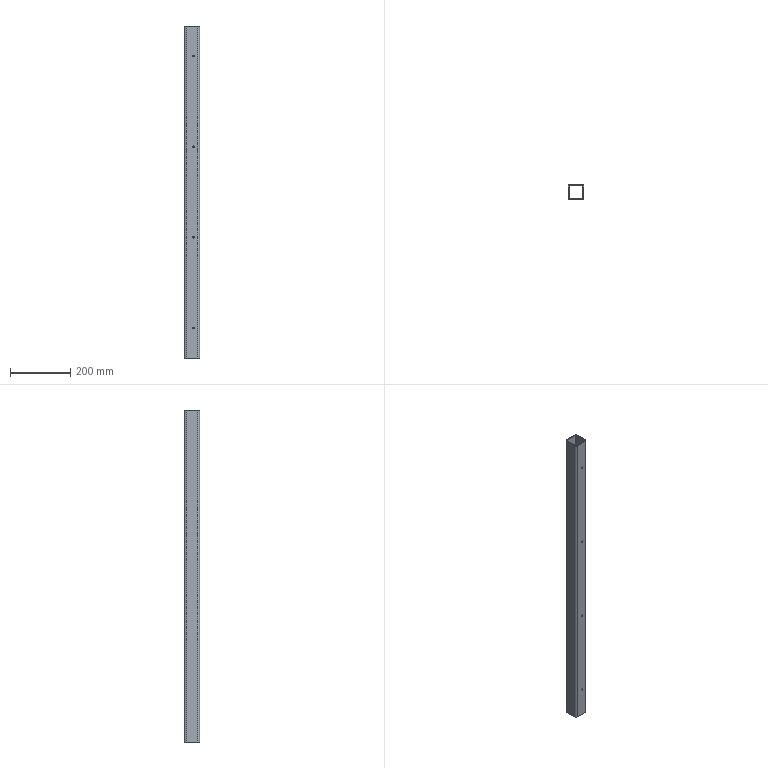Part | SolidWorks | features HoleWzd 1, WeldMemberFeat 1, WeldmentFeature 1 | 1 solid | 26 faces | box 50 x 50 x 1100 mm | volume 594670 mm3 | cylinder 16 | plane 10 | commonest cylinder face diameters 5 x8 6 x4 12 x4
STEP:
#1=CARTESIAN_POINT('',(5.,-22.,-102.5));
#2=VERTEX_POINT('',#1);
#3=CARTESIAN_POINT('',(5.,-22.,-97.5));
#4=VERTEX_POINT('',#3);
#5=CARTESIAN_POINT('',(5.,-22.,-100.));
#6=DIRECTION('',(0.,1.,0.));
#7=DIRECTION('',(0.,0.,1.));
#8=AXIS2_PLACEMENT_3D('',#5,#6,#7);
#9=CIRCLE('',#8,2.5);
#10=EDGE_CURVE('',#2,#4,#9,.T.);
#11=ORIENTED_EDGE('',*,*,#10,.T.);
#12=CARTESIAN_POINT('',(5.,-25.,-97.5));
#13=VERTEX_POINT('',#12);
#14=CARTESIAN_POINT('',(5.,-25.,-97.5));
#15=DIRECTION('',(0.,-1.,0.));
#16=VECTOR('',#15,1000.);
#17=LINE('',#14,#16);
#18=EDGE_CURVE('',#4,#13,#17,.T.);
#19=ORIENTED_EDGE('',*,*,#18,.T.);
#20=CARTESIAN_POINT('',(5.,-25.,-102.5));
#21=VERTEX_POINT('',#20);
#22=CARTESIAN_POINT('',(5.,-25.,-100.));
#23=DIRECTION('',(0.,-1.,0.));
#24=DIRECTION('',(0.,0.,-1.));
#25=AXIS2_PLACEMENT_3D('',#22,#23,#24);
#26=CIRCLE('',#25,2.5);
#27=EDGE_CURVE('',#13,#21,#26,.T.);
#28=ORIENTED_EDGE('',*,*,#27,.T.);
#29=CARTESIAN_POINT('',(5.,-25.,-102.5));
#30=DIRECTION('',(0.,-1.,0.));
#31=VECTOR('',#30,1000.);
#32=LINE('',#29,#31);
#33=EDGE_CURVE('',#2,#21,#32,.T.);
#34=ORIENTED_EDGE('',*,*,#33,.F.);
#35=EDGE_LOOP('',(#11,#19,#28,#34));
#36=FACE_OUTER_BOUND('',#35,.T.);
#37=CARTESIAN_POINT('',(5.,-25.,-100.));
#38=DIRECTION('',(0.,-1.,0.));
#39=DIRECTION('',(0.,0.,-1.));
#40=AXIS2_PLACEMENT_3D('',#37,#38,#39);
#41=CYLINDRICAL_SURFACE('',#40,2.5);
#42=ADVANCED_FACE('',(#36),#41,.F.);
#43=CARTESIAN_POINT('',(5.,-22.,-402.5));
#44=VERTEX_POINT('',#43);
#45=CARTESIAN_POINT('',(5.,-22.,-397.5));
#46=VERTEX_POINT('',#45);
#47=CARTESIAN_POINT('',(5.,-22.,-400.));
#48=DIRECTION('',(0.,1.,0.));
#49=DIRECTION('',(0.,0.,1.));
#50=AXIS2_PLACEMENT_3D('',#47,#48,#49);
#51=CIRCLE('',#50,2.5);
#52=EDGE_CURVE('',#44,#46,#51,.T.);
#53=ORIENTED_EDGE('',*,*,#52,.T.);
#54=CARTESIAN_POINT('',(5.,-25.,-397.5));
#55=VERTEX_POINT('',#54);
#56=CARTESIAN_POINT('',(5.,-25.,-397.5));
#57=DIRECTION('',(0.,-1.,0.));
#58=VECTOR('',#57,1000.);
#59=LINE('',#56,#58);
#60=EDGE_CURVE('',#46,#55,#59,.T.);
#61=ORIENTED_EDGE('',*,*,#60,.T.);
#62=CARTESIAN_POINT('',(5.,-25.,-402.5));
#63=VERTEX_POINT('',#62);
#64=CARTESIAN_POINT('',(5.,-25.,-400.));
#65=DIRECTION('',(0.,-1.,0.));
#66=DIRECTION('',(0.,0.,-1.));
#67=AXIS2_PLACEMENT_3D('',#64,#65,#66);
#68=CIRCLE('',#67,2.5);
#69=EDGE_CURVE('',#55,#63,#68,.T.);
#70=ORIENTED_EDGE('',*,*,#69,.T.);
#71=CARTESIAN_POINT('',(5.,-25.,-402.5));
#72=DIRECTION('',(0.,-1.,0.));
#73=VECTOR('',#72,1000.);
#74=LINE('',#71,#73);
#75=EDGE_CURVE('',#44,#63,#74,.T.);
#76=ORIENTED_EDGE('',*,*,#75,.F.);
#77=EDGE_LOOP('',(#53,#61,#70,#76));
#78=FACE_OUTER_BOUND('',#77,.T.);
#79=CARTESIAN_POINT('',(5.,-25.,-400.));
#80=DIRECTION('',(0.,-1.,0.));
#81=DIRECTION('',(0.,0.,-1.));
#82=AXIS2_PLACEMENT_3D('',#79,#80,#81);
#83=CYLINDRICAL_SURFACE('',#82,2.5);
#84=ADVANCED_FACE('',(#78),#83,.F.);
#85=CARTESIAN_POINT('',(5.,-22.,-702.5));
#86=VERTEX_POINT('',#85);
#87=CARTESIAN_POINT('',(5.,-22.,-697.5));
#88=VERTEX_POINT('',#87);
#89=CARTESIAN_POINT('',(5.,-22.,-700.));
#90=DIRECTION('',(0.,1.,0.));
#91=DIRECTION('',(0.,0.,1.));
#92=AXIS2_PLACEMENT_3D('',#89,#90,#91);
#93=CIRCLE('',#92,2.5);
#94=EDGE_CURVE('',#86,#88,#93,.T.);
#95=ORIENTED_EDGE('',*,*,#94,.T.);
#96=CARTESIAN_POINT('',(5.,-25.,-697.5));
#97=VERTEX_POINT('',#96);
#98=CARTESIAN_POINT('',(5.,-25.,-697.5));
#99=DIRECTION('',(0.,-1.,0.));
#100=VECTOR('',#99,1000.);
#101=LINE('',#98,#100);
#102=EDGE_CURVE('',#88,#97,#101,.T.);
#103=ORIENTED_EDGE('',*,*,#102,.T.);
#104=CARTESIAN_POINT('',(5.,-25.,-702.5));
#105=VERTEX_POINT('',#104);
#106=CARTESIAN_POINT('',(5.,-25.,-700.));
#107=DIRECTION('',(0.,-1.,0.));
#108=DIRECTION('',(0.,0.,-1.));
#109=AXIS2_PLACEMENT_3D('',#106,#107,#108);
#110=CIRCLE('',#109,2.5);
#111=EDGE_CURVE('',#97,#105,#110,.T.);
#112=ORIENTED_EDGE('',*,*,#111,.T.);
#113=CARTESIAN_POINT('',(5.,-25.,-702.5));
#114=DIRECTION('',(0.,-1.,0.));
#115=VECTOR('',#114,1000.);
#116=LINE('',#113,#115);
#117=EDGE_CURVE('',#86,#105,#116,.T.);
#118=ORIENTED_EDGE('',*,*,#117,.F.);
#119=EDGE_LOOP('',(#95,#103,#112,#118));
#120=FACE_OUTER_BOUND('',#119,.T.);
#121=CARTESIAN_POINT('',(5.,-25.,-700.));
#122=DIRECTION('',(0.,-1.,0.));
#123=DIRECTION('',(0.,0.,-1.));
#124=AXIS2_PLACEMENT_3D('',#121,#122,#123);
#125=CYLINDRICAL_SURFACE('',#124,2.5);
#126=ADVANCED_FACE('',(#120),#125,.F.);
#127=CARTESIAN_POINT('',(5.,-22.,-1002.5));
#128=VERTEX_POINT('',#127);
#129=CARTESIAN_POINT('',(5.,-22.,-997.5));
#130=VERTEX_POINT('',#129);
#131=CARTESIAN_POINT('',(5.,-22.,-1000.));
#132=DIRECTION('',(0.,1.,0.));
#133=DIRECTION('',(0.,0.,1.));
#134=AXIS2_PLACEMENT_3D('',#131,#132,#133);
#135=CIRCLE('',#134,2.5);
#136=EDGE_CURVE('',#128,#130,#135,.T.);
#137=ORIENTED_EDGE('',*,*,#136,.T.);
#138=CARTESIAN_POINT('',(5.,-25.,-997.5));
#139=VERTEX_POINT('',#138);
#140=CARTESIAN_POINT('',(5.,-25.,-997.5));
#141=DIRECTION('',(0.,-1.,0.));
#142=VECTOR('',#141,1000.);
#143=LINE('',#140,#142);
#144=EDGE_CURVE('',#130,#139,#143,.T.);
#145=ORIENTED_EDGE('',*,*,#144,.T.);
#146=CARTESIAN_POINT('',(5.,-25.,-1002.5));
#147=VERTEX_POINT('',#146);
#148=CARTESIAN_POINT('',(5.,-25.,-1000.));
#149=DIRECTION('',(0.,-1.,0.));
#150=DIRECTION('',(0.,0.,-1.));
#151=AXIS2_PLACEMENT_3D('',#148,#149,#150);
#152=CIRCLE('',#151,2.5);
#153=EDGE_CURVE('',#139,#147,#152,.T.);
#154=ORIENTED_EDGE('',*,*,#153,.T.);
#155=CARTESIAN_POINT('',(5.,-25.,-1002.5));
#156=DIRECTION('',(0.,-1.,0.));
#157=VECTOR('',#156,1000.);
#158=LINE('',#155,#157);
#159=EDGE_CURVE('',#128,#147,#158,.T.);
#160=ORIENTED_EDGE('',*,*,#159,.F.);
#161=EDGE_LOOP('',(#137,#145,#154,#160));
#162=FACE_OUTER_BOUND('',#161,.T.);
#163=CARTESIAN_POINT('',(5.,-25.,-1000.));
#164=DIRECTION('',(0.,-1.,0.));
#165=DIRECTION('',(0.,0.,-1.));
#166=AXIS2_PLACEMENT_3D('',#163,#164,#165);
#167=CYLINDRICAL_SURFACE('',#166,2.5);
#168=ADVANCED_FACE('',(#162),#167,.F.);
#169=CARTESIAN_POINT('',(-25.,19.,0.));
#170=VERTEX_POINT('',#169);
#171=CARTESIAN_POINT('',(-19.,25.,0.));
#172=VERTEX_POINT('',#171);
#173=CARTESIAN_POINT('',(-19.,19.,0.));
#174=DIRECTION('',(0.,0.,-1.));
#175=DIRECTION('',(-1.,0.,0.));
#176=AXIS2_PLACEMENT_3D('',#173,#174,#175);
#177=CIRCLE('',#176,6.);
#178=EDGE_CURVE('',#170,#172,#177,.T.);
#179=ORIENTED_EDGE('',*,*,#178,.T.);
#180=CARTESIAN_POINT('',(-19.,25.,-1100.));
#181=VERTEX_POINT('',#180);
#182=CARTESIAN_POINT('',(-19.,25.,-1100.));
#183=DIRECTION('',(0.,0.,1.));
#184=VECTOR('',#183,1000.);
#185=LINE('',#182,#184);
#186=EDGE_CURVE('',#181,#172,#185,.T.);
#187=ORIENTED_EDGE('',*,*,#186,.F.);
#188=CARTESIAN_POINT('',(-25.,19.,-1100.));
#189=VERTEX_POINT('',#188);
#190=CARTESIAN_POINT('',(-19.,19.,-1100.));
#191=DIRECTION('',(0.,0.,-1.));
#192=DIRECTION('',(-1.,0.,0.));
#193=AXIS2_PLACEMENT_3D('',#190,#191,#192);
#194=CIRCLE('',#193,6.);
#195=EDGE_CURVE('',#189,#181,#194,.T.);
#196=ORIENTED_EDGE('',*,*,#195,.F.);
#197=CARTESIAN_POINT('',(-25.,19.,-1100.));
#198=DIRECTION('',(0.,0.,1.));
#199=VECTOR('',#198,1000.);
#200=LINE('',#197,#199);
#201=EDGE_CURVE('',#189,#170,#200,.T.);
#202=ORIENTED_EDGE('',*,*,#201,.T.);
#203=EDGE_LOOP('',(#179,#187,#196,#202));
#204=FACE_OUTER_BOUND('',#203,.T.);
#205=CARTESIAN_POINT('',(-19.,19.,-1100.));
#206=DIRECTION('',(0.,0.,1.));
#207=DIRECTION('',(1.,0.,0.));
#208=AXIS2_PLACEMENT_3D('',#205,#206,#207);
#209=CYLINDRICAL_SURFACE('',#208,6.);
#210=ADVANCED_FACE('',(#204),#209,.T.);
#211=CARTESIAN_POINT('',(19.,25.,0.));
#212=VERTEX_POINT('',#211);
#213=CARTESIAN_POINT('',(-19.,25.,0.));
#214=DIRECTION('',(1.,0.,0.));
#215=VECTOR('',#214,1000.);
#216=LINE('',#213,#215);
#217=EDGE_CURVE('',#172,#212,#216,.T.);
#218=ORIENTED_EDGE('',*,*,#217,.T.);
#219=CARTESIAN_POINT('',(19.,25.,-1100.));
#220=VERTEX_POINT('',#219);
#221=CARTESIAN_POINT('',(19.,25.,-1100.));
#222=DIRECTION('',(0.,0.,1.));
#223=VECTOR('',#222,1000.);
#224=LINE('',#221,#223);
#225=EDGE_CURVE('',#220,#212,#224,.T.);
#226=ORIENTED_EDGE('',*,*,#225,.F.);
#227=CARTESIAN_POINT('',(-19.,25.,-1100.));
#228=DIRECTION('',(1.,0.,0.));
#229=VECTOR('',#228,1000.);
#230=LINE('',#227,#229);
#231=EDGE_CURVE('',#181,#220,#230,.T.);
#232=ORIENTED_EDGE('',*,*,#231,.F.);
#233=ORIENTED_EDGE('',*,*,#186,.T.);
#234=EDGE_LOOP('',(#218,#226,#232,#233));
#235=FACE_OUTER_BOUND('',#234,.T.);
#236=CARTESIAN_POINT('',(-19.,25.,-1100.));
#237=DIRECTION('',(0.,-1.,0.));
#238=DIRECTION('',(0.,0.,-1.));
#239=AXIS2_PLACEMENT_3D('',#236,#237,#238);
#240=PLANE('',#239);
#241=ADVANCED_FACE('',(#235),#240,.F.);
#242=CARTESIAN_POINT('',(25.,19.,0.));
#243=VERTEX_POINT('',#242);
#244=CARTESIAN_POINT('',(19.,19.,0.));
#245=DIRECTION('',(0.,0.,-1.));
#246=DIRECTION('',(-1.,0.,0.));
#247=AXIS2_PLACEMENT_3D('',#244,#245,#246);
#248=CIRCLE('',#247,6.);
#249=EDGE_CURVE('',#212,#243,#248,.T.);
#250=ORIENTED_EDGE('',*,*,#249,.T.);
#251=CARTESIAN_POINT('',(25.,19.,-1100.));
#252=VERTEX_POINT('',#251);
#253=CARTESIAN_POINT('',(25.,19.,-1100.));
#254=DIRECTION('',(0.,0.,1.));
#255=VECTOR('',#254,1000.);
#256=LINE('',#253,#255);
#257=EDGE_CURVE('',#252,#243,#256,.T.);
#258=ORIENTED_EDGE('',*,*,#257,.F.);
#259=CARTESIAN_POINT('',(19.,19.,-1100.));
#260=DIRECTION('',(0.,0.,-1.));
#261=DIRECTION('',(-1.,0.,0.));
#262=AXIS2_PLACEMENT_3D('',#259,#260,#261);
#263=CIRCLE('',#262,6.);
#264=EDGE_CURVE('',#220,#252,#263,.T.);
#265=ORIENTED_EDGE('',*,*,#264,.F.);
#266=ORIENTED_EDGE('',*,*,#225,.T.);
#267=EDGE_LOOP('',(#250,#258,#265,#266));
#268=FACE_OUTER_BOUND('',#267,.T.);
#269=CARTESIAN_POINT('',(19.,19.,-1100.));
#270=DIRECTION('',(0.,0.,1.));
#271=DIRECTION('',(1.,0.,0.));
#272=AXIS2_PLACEMENT_3D('',#269,#270,#271);
#273=CYLINDRICAL_SURFACE('',#272,6.);
#274=ADVANCED_FACE('',(#268),#273,.T.);
#275=CARTESIAN_POINT('',(25.,-19.,0.));
#276=VERTEX_POINT('',#275);
#277=CARTESIAN_POINT('',(25.,-19.,0.));
#278=DIRECTION('',(0.,-1.,0.));
#279=VECTOR('',#278,1000.);
#280=LINE('',#277,#279);
#281=EDGE_CURVE('',#243,#276,#280,.T.);
#282=ORIENTED_EDGE('',*,*,#281,.T.);
#283=CARTESIAN_POINT('',(25.,-19.,-1100.));
#284=VERTEX_POINT('',#283);
#285=CARTESIAN_POINT('',(25.,-19.,-1100.));
#286=DIRECTION('',(0.,0.,1.));
#287=VECTOR('',#286,1000.);
#288=LINE('',#285,#287);
#289=EDGE_CURVE('',#284,#276,#288,.T.);
#290=ORIENTED_EDGE('',*,*,#289,.F.);
#291=CARTESIAN_POINT('',(25.,-19.,-1100.));
#292=DIRECTION('',(0.,-1.,0.));
#293=VECTOR('',#292,1000.);
#294=LINE('',#291,#293);
#295=EDGE_CURVE('',#252,#284,#294,.T.);
#296=ORIENTED_EDGE('',*,*,#295,.F.);
#297=ORIENTED_EDGE('',*,*,#257,.T.);
#298=EDGE_LOOP('',(#282,#290,#296,#297));
#299=FACE_OUTER_BOUND('',#298,.T.);
#300=CARTESIAN_POINT('',(25.,-19.,-1100.));
#301=DIRECTION('',(-1.,0.,0.));
#302=DIRECTION('',(0.,0.,1.));
#303=AXIS2_PLACEMENT_3D('',#300,#301,#302);
#304=PLANE('',#303);
#305=ADVANCED_FACE('',(#299),#304,.F.);
#306=CARTESIAN_POINT('',(19.,-25.,0.));
#307=VERTEX_POINT('',#306);
#308=CARTESIAN_POINT('',(19.,-19.,0.));
#309=DIRECTION('',(0.,0.,-1.));
#310=DIRECTION('',(-1.,0.,0.));
#311=AXIS2_PLACEMENT_3D('',#308,#309,#310);
#312=CIRCLE('',#311,6.);
#313=EDGE_CURVE('',#276,#307,#312,.T.);
#314=ORIENTED_EDGE('',*,*,#313,.T.);
#315=CARTESIAN_POINT('',(19.,-25.,-1100.));
#316=VERTEX_POINT('',#315);
#317=CARTESIAN_POINT('',(19.,-25.,-1100.));
#318=DIRECTION('',(0.,0.,1.));
#319=VECTOR('',#318,1000.);
#320=LINE('',#317,#319);
#321=EDGE_CURVE('',#316,#307,#320,.T.);
#322=ORIENTED_EDGE('',*,*,#321,.F.);
#323=CARTESIAN_POINT('',(19.,-19.,-1100.));
#324=DIRECTION('',(0.,0.,-1.));
#325=DIRECTION('',(-1.,0.,0.));
#326=AXIS2_PLACEMENT_3D('',#323,#324,#325);
#327=CIRCLE('',#326,6.);
#328=EDGE_CURVE('',#284,#316,#327,.T.);
#329=ORIENTED_EDGE('',*,*,#328,.F.);
#330=ORIENTED_EDGE('',*,*,#289,.T.);
#331=EDGE_LOOP('',(#314,#322,#329,#330));
#332=FACE_OUTER_BOUND('',#331,.T.);
#333=CARTESIAN_POINT('',(19.,-19.,-1100.));
#334=DIRECTION('',(0.,0.,1.));
#335=DIRECTION('',(1.,0.,0.));
#336=AXIS2_PLACEMENT_3D('',#333,#334,#335);
#337=CYLINDRICAL_SURFACE('',#336,6.);
#338=ADVANCED_FACE('',(#332),#337,.T.);
#339=CARTESIAN_POINT('',(5.,-25.,-100.));
#340=DIRECTION('',(0.,-1.,0.));
#341=DIRECTION('',(0.,0.,-1.));
#342=AXIS2_PLACEMENT_3D('',#339,#340,#341);
#343=CIRCLE('',#342,2.5);
#344=EDGE_CURVE('',#21,#13,#343,.T.);
#345=ORIENTED_EDGE('',*,*,#344,.F.);
#346=ORIENTED_EDGE('',*,*,#27,.F.);
#347=EDGE_LOOP('',(#345,#346));
#348=FACE_BOUND('',#347,.T.);
#349=CARTESIAN_POINT('',(5.,-25.,-400.));
#350=DIRECTION('',(0.,-1.,0.));
#351=DIRECTION('',(0.,0.,-1.));
#352=AXIS2_PLACEMENT_3D('',#349,#350,#351);
#353=CIRCLE('',#352,2.5);
#354=EDGE_CURVE('',#63,#55,#353,.T.);
#355=ORIENTED_EDGE('',*,*,#354,.F.);
#356=ORIENTED_EDGE('',*,*,#69,.F.);
#357=EDGE_LOOP('',(#355,#356));
#358=FACE_BOUND('',#357,.T.);
#359=CARTESIAN_POINT('',(5.,-25.,-700.));
#360=DIRECTION('',(0.,-1.,0.));
#361=DIRECTION('',(0.,0.,-1.));
#362=AXIS2_PLACEMENT_3D('',#359,#360,#361);
#363=CIRCLE('',#362,2.5);
#364=EDGE_CURVE('',#105,#97,#363,.T.);
#365=ORIENTED_EDGE('',*,*,#364,.F.);
#366=ORIENTED_EDGE('',*,*,#111,.F.);
#367=EDGE_LOOP('',(#365,#366));
#368=FACE_BOUND('',#367,.T.);
#369=CARTESIAN_POINT('',(5.,-25.,-1000.));
#370=DIRECTION('',(0.,-1.,0.));
#371=DIRECTION('',(0.,0.,-1.));
#372=AXIS2_PLACEMENT_3D('',#369,#370,#371);
#373=CIRCLE('',#372,2.5);
#374=EDGE_CURVE('',#147,#139,#373,.T.);
#375=ORIENTED_EDGE('',*,*,#374,.F.);
#376=ORIENTED_EDGE('',*,*,#153,.F.);
#377=EDGE_LOOP('',(#375,#376));
#378=FACE_BOUND('',#377,.T.);
#379=CARTESIAN_POINT('',(-19.,-25.,0.));
#380=VERTEX_POINT('',#379);
#381=CARTESIAN_POINT('',(19.,-25.,0.));
#382=DIRECTION('',(-1.,0.,0.));
#383=VECTOR('',#382,1000.);
#384=LINE('',#381,#383);
#385=EDGE_CURVE('',#307,#380,#384,.T.);
#386=ORIENTED_EDGE('',*,*,#385,.T.);
#387=CARTESIAN_POINT('',(-19.,-25.,-1100.));
#388=VERTEX_POINT('',#387);
#389=CARTESIAN_POINT('',(-19.,-25.,-1100.));
#390=DIRECTION('',(0.,0.,1.));
#391=VECTOR('',#390,1000.);
#392=LINE('',#389,#391);
#393=EDGE_CURVE('',#388,#380,#392,.T.);
#394=ORIENTED_EDGE('',*,*,#393,.F.);
#395=CARTESIAN_POINT('',(19.,-25.,-1100.));
#396=DIRECTION('',(-1.,0.,0.));
#397=VECTOR('',#396,1000.);
#398=LINE('',#395,#397);
#399=EDGE_CURVE('',#316,#388,#398,.T.);
#400=ORIENTED_EDGE('',*,*,#399,.F.);
#401=ORIENTED_EDGE('',*,*,#321,.T.);
#402=EDGE_LOOP('',(#386,#394,#400,#401));
#403=FACE_OUTER_BOUND('',#402,.T.);
#404=CARTESIAN_POINT('',(19.,-25.,-1100.));
#405=DIRECTION('',(0.,1.,0.));
#406=DIRECTION('',(0.,0.,1.));
#407=AXIS2_PLACEMENT_3D('',#404,#405,#406);
#408=PLANE('',#407);
#409=ADVANCED_FACE('',(#348,#358,#368,#378,#403),#408,.F.);
#410=CARTESIAN_POINT('',(-25.,-19.,0.));
#411=VERTEX_POINT('',#410);
#412=CARTESIAN_POINT('',(-19.,-19.,0.));
#413=DIRECTION('',(0.,0.,-1.));
#414=DIRECTION('',(-1.,0.,0.));
#415=AXIS2_PLACEMENT_3D('',#412,#413,#414);
#416=CIRCLE('',#415,6.);
#417=EDGE_CURVE('',#380,#411,#416,.T.);
#418=ORIENTED_EDGE('',*,*,#417,.T.);
#419=CARTESIAN_POINT('',(-25.,-19.,-1100.));
#420=VERTEX_POINT('',#419);
#421=CARTESIAN_POINT('',(-25.,-19.,-1100.));
#422=DIRECTION('',(0.,0.,1.));
#423=VECTOR('',#422,1000.);
#424=LINE('',#421,#423);
#425=EDGE_CURVE('',#420,#411,#424,.T.);
#426=ORIENTED_EDGE('',*,*,#425,.F.);
#427=CARTESIAN_POINT('',(-19.,-19.,-1100.));
#428=DIRECTION('',(0.,0.,-1.));
#429=DIRECTION('',(-1.,0.,0.));
#430=AXIS2_PLACEMENT_3D('',#427,#428,#429);
#431=CIRCLE('',#430,6.);
#432=EDGE_CURVE('',#388,#420,#431,.T.);
#433=ORIENTED_EDGE('',*,*,#432,.F.);
#434=ORIENTED_EDGE('',*,*,#393,.T.);
#435=EDGE_LOOP('',(#418,#426,#433,#434));
#436=FACE_OUTER_BOUND('',#435,.T.);
#437=CARTESIAN_POINT('',(-19.,-19.,-1100.));
#438=DIRECTION('',(0.,0.,1.));
#439=DIRECTION('',(1.,0.,0.));
#440=AXIS2_PLACEMENT_3D('',#437,#438,#439);
#441=CYLINDRICAL_SURFACE('',#440,6.);
#442=ADVANCED_FACE('',(#436),#441,.T.);
#443=CARTESIAN_POINT('',(19.,22.,0.));
#444=VERTEX_POINT('',#443);
#445=CARTESIAN_POINT('',(22.,19.,0.));
#446=VERTEX_POINT('',#445);
#447=CARTESIAN_POINT('',(19.,19.,0.));
#448=DIRECTION('',(0.,0.,-1.));
#449=DIRECTION('',(-1.,0.,0.));
#450=AXIS2_PLACEMENT_3D('',#447,#448,#449);
#451=CIRCLE('',#450,3.);
#452=EDGE_CURVE('',#444,#446,#451,.T.);
#453=ORIENTED_EDGE('',*,*,#452,.F.);
#454=CARTESIAN_POINT('',(19.,22.,-1100.));
#455=VERTEX_POINT('',#454);
#456=CARTESIAN_POINT('',(19.,22.,-1100.));
#457=DIRECTION('',(0.,0.,1.));
#458=VECTOR('',#457,1000.);
#459=LINE('',#456,#458);
#460=EDGE_CURVE('',#455,#444,#459,.T.);
#461=ORIENTED_EDGE('',*,*,#460,.F.);
#462=CARTESIAN_POINT('',(22.,19.,-1100.));
#463=VERTEX_POINT('',#462);
#464=CARTESIAN_POINT('',(19.,19.,-1100.));
#465=DIRECTION('',(0.,0.,-1.));
#466=DIRECTION('',(-1.,0.,0.));
#467=AXIS2_PLACEMENT_3D('',#464,#465,#466);
#468=CIRCLE('',#467,3.);
#469=EDGE_CURVE('',#455,#463,#468,.T.);
#470=ORIENTED_EDGE('',*,*,#469,.T.);
#471=CARTESIAN_POINT('',(22.,19.,-1100.));
#472=DIRECTION('',(0.,0.,1.));
#473=VECTOR('',#472,1000.);
#474=LINE('',#471,#473);
#475=EDGE_CURVE('',#463,#446,#474,.T.);
#476=ORIENTED_EDGE('',*,*,#475,.T.);
#477=EDGE_LOOP('',(#453,#461,#470,#476));
#478=FACE_OUTER_BOUND('',#477,.T.);
#479=CARTESIAN_POINT('',(19.,19.,-1100.));
#480=DIRECTION('',(0.,0.,1.));
#481=DIRECTION('',(1.,0.,0.));
#482=AXIS2_PLACEMENT_3D('',#479,#480,#481);
#483=CYLINDRICAL_SURFACE('',#482,3.);
#484=ADVANCED_FACE('',(#478),#483,.F.);
#485=CARTESIAN_POINT('',(-19.,22.,0.));
#486=VERTEX_POINT('',#485);
#487=CARTESIAN_POINT('',(-19.,22.,0.));
#488=DIRECTION('',(1.,0.,0.));
#489=VECTOR('',#488,1000.);
#490=LINE('',#487,#489);
#491=EDGE_CURVE('',#486,#444,#490,.T.);
#492=ORIENTED_EDGE('',*,*,#491,.F.);
#493=CARTESIAN_POINT('',(-19.,22.,-1100.));
#494=VERTEX_POINT('',#493);
#495=CARTESIAN_POINT('',(-19.,22.,-1100.));
#496=DIRECTION('',(0.,0.,1.));
#497=VECTOR('',#496,1000.);
#498=LINE('',#495,#497);
#499=EDGE_CURVE('',#494,#486,#498,.T.);
#500=ORIENTED_EDGE('',*,*,#499,.F.);
#501=CARTESIAN_POINT('',(-19.,22.,-1100.));
#502=DIRECTION('',(1.,0.,0.));
#503=VECTOR('',#502,1000.);
#504=LINE('',#501,#503);
#505=EDGE_CURVE('',#494,#455,#504,.T.);
#506=ORIENTED_EDGE('',*,*,#505,.T.);
#507=ORIENTED_EDGE('',*,*,#460,.T.);
#508=EDGE_LOOP('',(#492,#500,#506,#507));
#509=FACE_OUTER_BOUND('',#508,.T.);
#510=CARTESIAN_POINT('',(-19.,22.,-1100.));
#511=DIRECTION('',(0.,-1.,0.));
#512=DIRECTION('',(0.,0.,-1.));
#513=AXIS2_PLACEMENT_3D('',#510,#511,#512);
#514=PLANE('',#513);
#515=ADVANCED_FACE('',(#509),#514,.T.);
#516=CARTESIAN_POINT('',(-22.,19.,0.));
#517=VERTEX_POINT('',#516);
#518=CARTESIAN_POINT('',(-19.,19.,0.));
#519=DIRECTION('',(0.,0.,-1.));
#520=DIRECTION('',(-1.,0.,0.));
#521=AXIS2_PLACEMENT_3D('',#518,#519,#520);
#522=CIRCLE('',#521,3.);
#523=EDGE_CURVE('',#517,#486,#522,.T.);
#524=ORIENTED_EDGE('',*,*,#523,.F.);
#525=CARTESIAN_POINT('',(-22.,19.,-1100.));
#526=VERTEX_POINT('',#525);
#527=CARTESIAN_POINT('',(-22.,19.,-1100.));
#528=DIRECTION('',(0.,0.,1.));
#529=VECTOR('',#528,1000.);
#530=LINE('',#527,#529);
#531=EDGE_CURVE('',#526,#517,#530,.T.);
#532=ORIENTED_EDGE('',*,*,#531,.F.);
#533=CARTESIAN_POINT('',(-19.,19.,-1100.));
#534=DIRECTION('',(0.,0.,-1.));
#535=DIRECTION('',(-1.,0.,0.));
#536=AXIS2_PLACEMENT_3D('',#533,#534,#535);
#537=CIRCLE('',#536,3.);
#538=EDGE_CURVE('',#526,#494,#537,.T.);
#539=ORIENTED_EDGE('',*,*,#538,.T.);
#540=ORIENTED_EDGE('',*,*,#499,.T.);
#541=EDGE_LOOP('',(#524,#532,#539,#540));
#542=FACE_OUTER_BOUND('',#541,.T.);
#543=CARTESIAN_POINT('',(-19.,19.,-1100.));
#544=DIRECTION('',(0.,0.,1.));
#545=DIRECTION('',(1.,0.,0.));
#546=AXIS2_PLACEMENT_3D('',#543,#544,#545);
#547=CYLINDRICAL_SURFACE('',#546,3.);
#548=ADVANCED_FACE('',(#542),#547,.F.);
#549=CARTESIAN_POINT('',(-22.,-19.,0.));
#550=VERTEX_POINT('',#549);
#551=CARTESIAN_POINT('',(-22.,19.,0.));
#552=DIRECTION('',(0.,1.,0.));
#553=VECTOR('',#552,1000.);
#554=LINE('',#551,#553);
#555=EDGE_CURVE('',#550,#517,#554,.T.);
#556=ORIENTED_EDGE('',*,*,#555,.F.);
#557=CARTESIAN_POINT('',(-22.,-19.,-1100.));
#558=VERTEX_POINT('',#557);
#559=CARTESIAN_POINT('',(-22.,-19.,-1100.));
#560=DIRECTION('',(0.,0.,1.));
#561=VECTOR('',#560,1000.);
#562=LINE('',#559,#561);
#563=EDGE_CURVE('',#558,#550,#562,.T.);
#564=ORIENTED_EDGE('',*,*,#563,.F.);
#565=CARTESIAN_POINT('',(-22.,19.,-1100.));
#566=DIRECTION('',(0.,1.,0.));
#567=VECTOR('',#566,1000.);
#568=LINE('',#565,#567);
#569=EDGE_CURVE('',#558,#526,#568,.T.);
#570=ORIENTED_EDGE('',*,*,#569,.T.);
#571=ORIENTED_EDGE('',*,*,#531,.T.);
#572=EDGE_LOOP('',(#556,#564,#570,#571));
#573=FACE_OUTER_BOUND('',#572,.T.);
#574=CARTESIAN_POINT('',(-22.,19.,-1100.));
#575=DIRECTION('',(1.,0.,0.));
#576=DIRECTION('',(0.,0.,-1.));
#577=AXIS2_PLACEMENT_3D('',#574,#575,#576);
#578=PLANE('',#577);
#579=ADVANCED_FACE('',(#573),#578,.T.);
#580=CARTESIAN_POINT('',(-19.,-22.,0.));
#581=VERTEX_POINT('',#580);
#582=CARTESIAN_POINT('',(-19.,-19.,0.));
#583=DIRECTION('',(0.,0.,-1.));
#584=DIRECTION('',(-1.,0.,0.));
#585=AXIS2_PLACEMENT_3D('',#582,#583,#584);
#586=CIRCLE('',#585,3.);
#587=EDGE_CURVE('',#581,#550,#586,.T.);
#588=ORIENTED_EDGE('',*,*,#587,.F.);
#589=CARTESIAN_POINT('',(-19.,-22.,-1100.));
#590=VERTEX_POINT('',#589);
#591=CARTESIAN_POINT('',(-19.,-22.,-1100.));
#592=DIRECTION('',(0.,0.,1.));
#593=VECTOR('',#592,1000.);
#594=LINE('',#591,#593);
#595=EDGE_CURVE('',#590,#581,#594,.T.);
#596=ORIENTED_EDGE('',*,*,#595,.F.);
#597=CARTESIAN_POINT('',(-19.,-19.,-1100.));
#598=DIRECTION('',(0.,0.,-1.));
#599=DIRECTION('',(-1.,0.,0.));
#600=AXIS2_PLACEMENT_3D('',#597,#598,#599);
#601=CIRCLE('',#600,3.);
#602=EDGE_CURVE('',#590,#558,#601,.T.);
#603=ORIENTED_EDGE('',*,*,#602,.T.);
#604=ORIENTED_EDGE('',*,*,#563,.T.);
#605=EDGE_LOOP('',(#588,#596,#603,#604));
#606=FACE_OUTER_BOUND('',#605,.T.);
#607=CARTESIAN_POINT('',(-19.,-19.,-1100.));
#608=DIRECTION('',(0.,0.,1.));
#609=DIRECTION('',(1.,0.,0.));
#610=AXIS2_PLACEMENT_3D('',#607,#608,#609);
#611=CYLINDRICAL_SURFACE('',#610,3.);
#612=ADVANCED_FACE('',(#606),#611,.F.);
#613=ORIENTED_EDGE('',*,*,#10,.F.);
#614=CARTESIAN_POINT('',(5.,-22.,-100.));
#615=DIRECTION('',(0.,1.,0.));
#616=DIRECTION('',(0.,0.,1.));
#617=AXIS2_PLACEMENT_3D('',#614,#615,#616);
#618=CIRCLE('',#617,2.5);
#619=EDGE_CURVE('',#4,#2,#618,.T.);
#620=ORIENTED_EDGE('',*,*,#619,.F.);
#621=EDGE_LOOP('',(#613,#620));
#622=FACE_BOUND('',#621,.T.);
#623=ORIENTED_EDGE('',*,*,#52,.F.);
#624=CARTESIAN_POINT('',(5.,-22.,-400.));
#625=DIRECTION('',(0.,1.,0.));
#626=DIRECTION('',(0.,0.,1.));
#627=AXIS2_PLACEMENT_3D('',#624,#625,#626);
#628=CIRCLE('',#627,2.5);
#629=EDGE_CURVE('',#46,#44,#628,.T.);
#630=ORIENTED_EDGE('',*,*,#629,.F.);
#631=EDGE_LOOP('',(#623,#630));
#632=FACE_BOUND('',#631,.T.);
#633=ORIENTED_EDGE('',*,*,#94,.F.);
#634=CARTESIAN_POINT('',(5.,-22.,-700.));
#635=DIRECTION('',(0.,1.,0.));
#636=DIRECTION('',(0.,0.,1.));
#637=AXIS2_PLACEMENT_3D('',#634,#635,#636);
#638=CIRCLE('',#637,2.5);
#639=EDGE_CURVE('',#88,#86,#638,.T.);
#640=ORIENTED_EDGE('',*,*,#639,.F.);
#641=EDGE_LOOP('',(#633,#640));
#642=FACE_BOUND('',#641,.T.);
#643=ORIENTED_EDGE('',*,*,#136,.F.);
#644=CARTESIAN_POINT('',(5.,-22.,-1000.));
#645=DIRECTION('',(0.,1.,0.));
#646=DIRECTION('',(0.,0.,1.));
#647=AXIS2_PLACEMENT_3D('',#644,#645,#646);
#648=CIRCLE('',#647,2.5);
#649=EDGE_CURVE('',#130,#128,#648,.T.);
#650=ORIENTED_EDGE('',*,*,#649,.F.);
#651=EDGE_LOOP('',(#643,#650));
#652=FACE_BOUND('',#651,.T.);
#653=CARTESIAN_POINT('',(19.,-22.,0.));
#654=VERTEX_POINT('',#653);
#655=CARTESIAN_POINT('',(19.,-22.,0.));
#656=DIRECTION('',(-1.,0.,0.));
#657=VECTOR('',#656,1000.);
#658=LINE('',#655,#657);
#659=EDGE_CURVE('',#654,#581,#658,.T.);
#660=ORIENTED_EDGE('',*,*,#659,.F.);
#661=CARTESIAN_POINT('',(19.,-22.,-1100.));
#662=VERTEX_POINT('',#661);
#663=CARTESIAN_POINT('',(19.,-22.,-1100.));
#664=DIRECTION('',(0.,0.,1.));
#665=VECTOR('',#664,1000.);
#666=LINE('',#663,#665);
#667=EDGE_CURVE('',#662,#654,#666,.T.);
#668=ORIENTED_EDGE('',*,*,#667,.F.);
#669=CARTESIAN_POINT('',(19.,-22.,-1100.));
#670=DIRECTION('',(-1.,0.,0.));
#671=VECTOR('',#670,1000.);
#672=LINE('',#669,#671);
#673=EDGE_CURVE('',#662,#590,#672,.T.);
#674=ORIENTED_EDGE('',*,*,#673,.T.);
#675=ORIENTED_EDGE('',*,*,#595,.T.);
#676=EDGE_LOOP('',(#660,#668,#674,#675));
#677=FACE_OUTER_BOUND('',#676,.T.);
#678=CARTESIAN_POINT('',(19.,-22.,-1100.));
#679=DIRECTION('',(0.,1.,0.));
#680=DIRECTION('',(0.,0.,1.));
#681=AXIS2_PLACEMENT_3D('',#678,#679,#680);
#682=PLANE('',#681);
#683=ADVANCED_FACE('',(#622,#632,#642,#652,#677),#682,.T.);
#684=CARTESIAN_POINT('',(22.,-19.,0.));
#685=VERTEX_POINT('',#684);
#686=CARTESIAN_POINT('',(19.,-19.,0.));
#687=DIRECTION('',(0.,0.,-1.));
#688=DIRECTION('',(-1.,0.,0.));
#689=AXIS2_PLACEMENT_3D('',#686,#687,#688);
#690=CIRCLE('',#689,3.);
#691=EDGE_CURVE('',#685,#654,#690,.T.);
#692=ORIENTED_EDGE('',*,*,#691,.F.);
#693=CARTESIAN_POINT('',(22.,-19.,-1100.));
#694=VERTEX_POINT('',#693);
#695=CARTESIAN_POINT('',(22.,-19.,-1100.));
#696=DIRECTION('',(0.,0.,1.));
#697=VECTOR('',#696,1000.);
#698=LINE('',#695,#697);
#699=EDGE_CURVE('',#694,#685,#698,.T.);
#700=ORIENTED_EDGE('',*,*,#699,.F.);
#701=CARTESIAN_POINT('',(19.,-19.,-1100.));
#702=DIRECTION('',(0.,0.,-1.));
#703=DIRECTION('',(-1.,0.,0.));
#704=AXIS2_PLACEMENT_3D('',#701,#702,#703);
#705=CIRCLE('',#704,3.);
#706=EDGE_CURVE('',#694,#662,#705,.T.);
#707=ORIENTED_EDGE('',*,*,#706,.T.);
#708=ORIENTED_EDGE('',*,*,#667,.T.);
#709=EDGE_LOOP('',(#692,#700,#707,#708));
#710=FACE_OUTER_BOUND('',#709,.T.);
#711=CARTESIAN_POINT('',(19.,-19.,-1100.));
#712=DIRECTION('',(0.,0.,1.));
#713=DIRECTION('',(1.,0.,0.));
#714=AXIS2_PLACEMENT_3D('',#711,#712,#713);
#715=CYLINDRICAL_SURFACE('',#714,3.);
#716=ADVANCED_FACE('',(#710),#715,.F.);
#717=CARTESIAN_POINT('',(22.,-19.,0.));
#718=DIRECTION('',(0.,-1.,0.));
#719=VECTOR('',#718,1000.);
#720=LINE('',#717,#719);
#721=EDGE_CURVE('',#446,#685,#720,.T.);
#722=ORIENTED_EDGE('',*,*,#721,.F.);
#723=ORIENTED_EDGE('',*,*,#475,.F.);
#724=CARTESIAN_POINT('',(22.,-19.,-1100.));
#725=DIRECTION('',(0.,-1.,0.));
#726=VECTOR('',#725,1000.);
#727=LINE('',#724,#726);
#728=EDGE_CURVE('',#463,#694,#727,.T.);
#729=ORIENTED_EDGE('',*,*,#728,.T.);
#730=ORIENTED_EDGE('',*,*,#699,.T.);
#731=EDGE_LOOP('',(#722,#723,#729,#730));
#732=FACE_OUTER_BOUND('',#731,.T.);
#733=CARTESIAN_POINT('',(22.,-19.,-1100.));
#734=DIRECTION('',(-1.,0.,0.));
#735=DIRECTION('',(0.,0.,1.));
#736=AXIS2_PLACEMENT_3D('',#733,#734,#735);
#737=PLANE('',#736);
#738=ADVANCED_FACE('',(#732),#737,.T.);
#739=CARTESIAN_POINT('',(-25.,19.,0.));
#740=DIRECTION('',(0.,1.,0.));
#741=VECTOR('',#740,1000.);
#742=LINE('',#739,#741);
#743=EDGE_CURVE('',#411,#170,#742,.T.);
#744=ORIENTED_EDGE('',*,*,#743,.T.);
#745=ORIENTED_EDGE('',*,*,#201,.F.);
#746=CARTESIAN_POINT('',(-25.,19.,-1100.));
#747=DIRECTION('',(0.,1.,0.));
#748=VECTOR('',#747,1000.);
#749=LINE('',#746,#748);
#750=EDGE_CURVE('',#420,#189,#749,.T.);
#751=ORIENTED_EDGE('',*,*,#750,.F.);
#752=ORIENTED_EDGE('',*,*,#425,.T.);
#753=EDGE_LOOP('',(#744,#745,#751,#752));
#754=FACE_OUTER_BOUND('',#753,.T.);
#755=CARTESIAN_POINT('',(-25.,19.,-1100.));
#756=DIRECTION('',(1.,0.,0.));
#757=DIRECTION('',(0.,0.,-1.));
#758=AXIS2_PLACEMENT_3D('',#755,#756,#757);
#759=PLANE('',#758);
#760=ADVANCED_FACE('',(#754),#759,.F.);
#761=ORIENTED_EDGE('',*,*,#469,.F.);
#762=ORIENTED_EDGE('',*,*,#505,.F.);
#763=ORIENTED_EDGE('',*,*,#538,.F.);
#764=ORIENTED_EDGE('',*,*,#569,.F.);
#765=ORIENTED_EDGE('',*,*,#602,.F.);
#766=ORIENTED_EDGE('',*,*,#673,.F.);
#767=ORIENTED_EDGE('',*,*,#706,.F.);
#768=ORIENTED_EDGE('',*,*,#728,.F.);
#769=EDGE_LOOP('',(#761,#762,#763,#764,#765,#766,#767,#768));
#770=FACE_BOUND('',#769,.T.);
#771=ORIENTED_EDGE('',*,*,#195,.T.);
#772=ORIENTED_EDGE('',*,*,#231,.T.);
#773=ORIENTED_EDGE('',*,*,#264,.T.);
#774=ORIENTED_EDGE('',*,*,#295,.T.);
#775=ORIENTED_EDGE('',*,*,#328,.T.);
#776=ORIENTED_EDGE('',*,*,#399,.T.);
#777=ORIENTED_EDGE('',*,*,#432,.T.);
#778=ORIENTED_EDGE('',*,*,#750,.T.);
#779=EDGE_LOOP('',(#771,#772,#773,#774,#775,#776,#777,#778));
#780=FACE_OUTER_BOUND('',#779,.T.);
#781=CARTESIAN_POINT('',(-19.,19.,-1100.));
#782=DIRECTION('',(0.,0.,-1.));
#783=DIRECTION('',(-1.,0.,0.));
#784=AXIS2_PLACEMENT_3D('',#781,#782,#783);
#785=PLANE('',#784);
#786=ADVANCED_FACE('',(#770,#780),#785,.T.);
#787=ORIENTED_EDGE('',*,*,#452,.T.);
#788=ORIENTED_EDGE('',*,*,#721,.T.);
#789=ORIENTED_EDGE('',*,*,#691,.T.);
#790=ORIENTED_EDGE('',*,*,#659,.T.);
#791=ORIENTED_EDGE('',*,*,#587,.T.);
#792=ORIENTED_EDGE('',*,*,#555,.T.);
#793=ORIENTED_EDGE('',*,*,#523,.T.);
#794=ORIENTED_EDGE('',*,*,#491,.T.);
#795=EDGE_LOOP('',(#787,#788,#789,#790,#791,#792,#793,#794));
#796=FACE_BOUND('',#795,.T.);
#797=ORIENTED_EDGE('',*,*,#178,.F.);
#798=ORIENTED_EDGE('',*,*,#743,.F.);
#799=ORIENTED_EDGE('',*,*,#417,.F.);
#800=ORIENTED_EDGE('',*,*,#385,.F.);
#801=ORIENTED_EDGE('',*,*,#313,.F.);
#802=ORIENTED_EDGE('',*,*,#281,.F.);
#803=ORIENTED_EDGE('',*,*,#249,.F.);
#804=ORIENTED_EDGE('',*,*,#217,.F.);
#805=EDGE_LOOP('',(#797,#798,#799,#800,#801,#802,#803,#804));
#806=FACE_OUTER_BOUND('',#805,.T.);
#807=CARTESIAN_POINT('',(-19.,19.,0.));
#808=DIRECTION('',(0.,0.,-1.));
#809=DIRECTION('',(-1.,0.,0.));
#810=AXIS2_PLACEMENT_3D('',#807,#808,#809);
#811=PLANE('',#810);
#812=ADVANCED_FACE('',(#796,#806),#811,.F.);
#813=ORIENTED_EDGE('',*,*,#144,.F.);
#814=ORIENTED_EDGE('',*,*,#649,.T.);
#815=ORIENTED_EDGE('',*,*,#159,.T.);
#816=ORIENTED_EDGE('',*,*,#374,.T.);
#817=EDGE_LOOP('',(#813,#814,#815,#816));
#818=FACE_OUTER_BOUND('',#817,.T.);
#819=CARTESIAN_POINT('',(5.,-25.,-1000.));
#820=DIRECTION('',(0.,-1.,0.));
#821=DIRECTION('',(0.,0.,-1.));
#822=AXIS2_PLACEMENT_3D('',#819,#820,#821);
#823=CYLINDRICAL_SURFACE('',#822,2.5);
#824=ADVANCED_FACE('',(#818),#823,.F.);
#825=ORIENTED_EDGE('',*,*,#102,.F.);
#826=ORIENTED_EDGE('',*,*,#639,.T.);
#827=ORIENTED_EDGE('',*,*,#117,.T.);
#828=ORIENTED_EDGE('',*,*,#364,.T.);
#829=EDGE_LOOP('',(#825,#826,#827,#828));
#830=FACE_OUTER_BOUND('',#829,.T.);
#831=CARTESIAN_POINT('',(5.,-25.,-700.));
#832=DIRECTION('',(0.,-1.,0.));
#833=DIRECTION('',(0.,0.,-1.));
#834=AXIS2_PLACEMENT_3D('',#831,#832,#833);
#835=CYLINDRICAL_SURFACE('',#834,2.5);
#836=ADVANCED_FACE('',(#830),#835,.F.);
#837=ORIENTED_EDGE('',*,*,#60,.F.);
#838=ORIENTED_EDGE('',*,*,#629,.T.);
#839=ORIENTED_EDGE('',*,*,#75,.T.);
#840=ORIENTED_EDGE('',*,*,#354,.T.);
#841=EDGE_LOOP('',(#837,#838,#839,#840));
#842=FACE_OUTER_BOUND('',#841,.T.);
#843=CARTESIAN_POINT('',(5.,-25.,-400.));
#844=DIRECTION('',(0.,-1.,0.));
#845=DIRECTION('',(0.,0.,-1.));
#846=AXIS2_PLACEMENT_3D('',#843,#844,#845);
#847=CYLINDRICAL_SURFACE('',#846,2.5);
#848=ADVANCED_FACE('',(#842),#847,.F.);
#849=ORIENTED_EDGE('',*,*,#18,.F.);
#850=ORIENTED_EDGE('',*,*,#619,.T.);
#851=ORIENTED_EDGE('',*,*,#33,.T.);
#852=ORIENTED_EDGE('',*,*,#344,.T.);
#853=EDGE_LOOP('',(#849,#850,#851,#852));
#854=FACE_OUTER_BOUND('',#853,.T.);
#855=CARTESIAN_POINT('',(5.,-25.,-100.));
#856=DIRECTION('',(0.,-1.,0.));
#857=DIRECTION('',(0.,0.,-1.));
#858=AXIS2_PLACEMENT_3D('',#855,#856,#857);
#859=CYLINDRICAL_SURFACE('',#858,2.5);
#860=ADVANCED_FACE('',(#854),#859,.F.);
#861=CLOSED_SHELL('',(#42,#84,#126,#168,#210,#241,#274,#305,#338,#409,#442,#484,#515,#548,#579,#612,#683,#716,#738,#760,#786,#812,#824,#836,#848,#860));
#862=MANIFOLD_SOLID_BREP('',#861);
#863=CARTESIAN_POINT('',(0.,0.,0.));
#864=DIRECTION('',(0.,0.,1.));
#865=DIRECTION('',(1.,0.,0.));
#866=AXIS2_PLACEMENT_3D('',#863,#864,#865);
#867=(LENGTH_UNIT()NAMED_UNIT(*)SI_UNIT(.MILLI.,.METRE.));
#868=UNCERTAINTY_MEASURE_WITH_UNIT(LENGTH_MEASURE(0.00001),#867,'','');
#869=(NAMED_UNIT(*)PLANE_ANGLE_UNIT()SI_UNIT($,.RADIAN.));
#870=(NAMED_UNIT(*)SI_UNIT($,.STERADIAN.)SOLID_ANGLE_UNIT());
#871=(GEOMETRIC_REPRESENTATION_CONTEXT(3)GLOBAL_UNCERTAINTY_ASSIGNED_CONTEXT((#868))GLOBAL_UNIT_ASSIGNED_CONTEXT((#867,#869,#870))REPRESENTATION_CONTEXT('',''));
#872=ADVANCED_BREP_SHAPE_REPRESENTATION('',(#862,#866),#871);